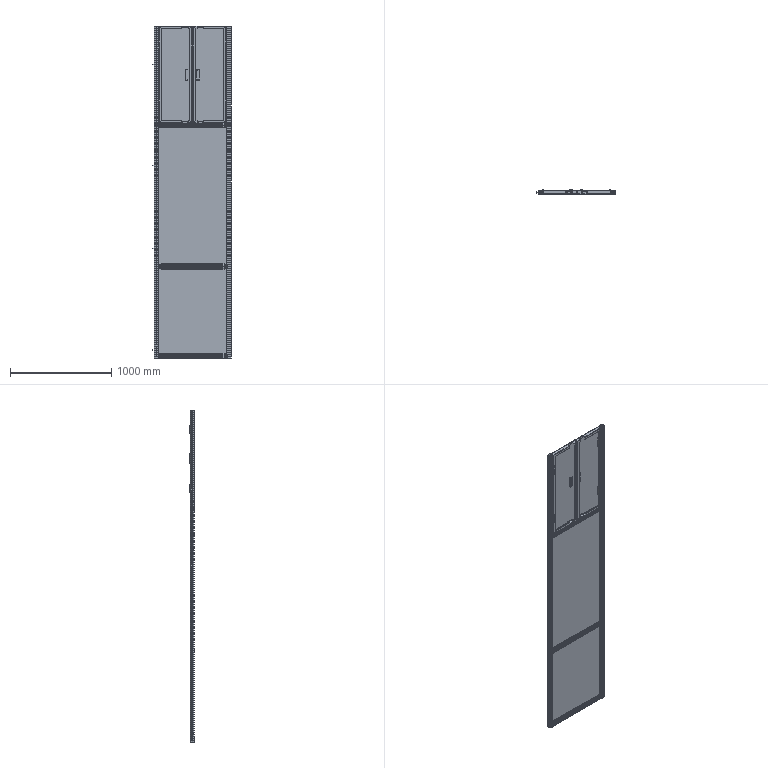Part | SolidWorks | 99 solids | 3616 faces | volume 15444382 mm3 | plane 2225 | cylinder 1015 | cone 284 | spline 92 | commonest cylinder face diameters 6.8 x127 8 x76 5 x68 2 x62 4 x60 10 x48